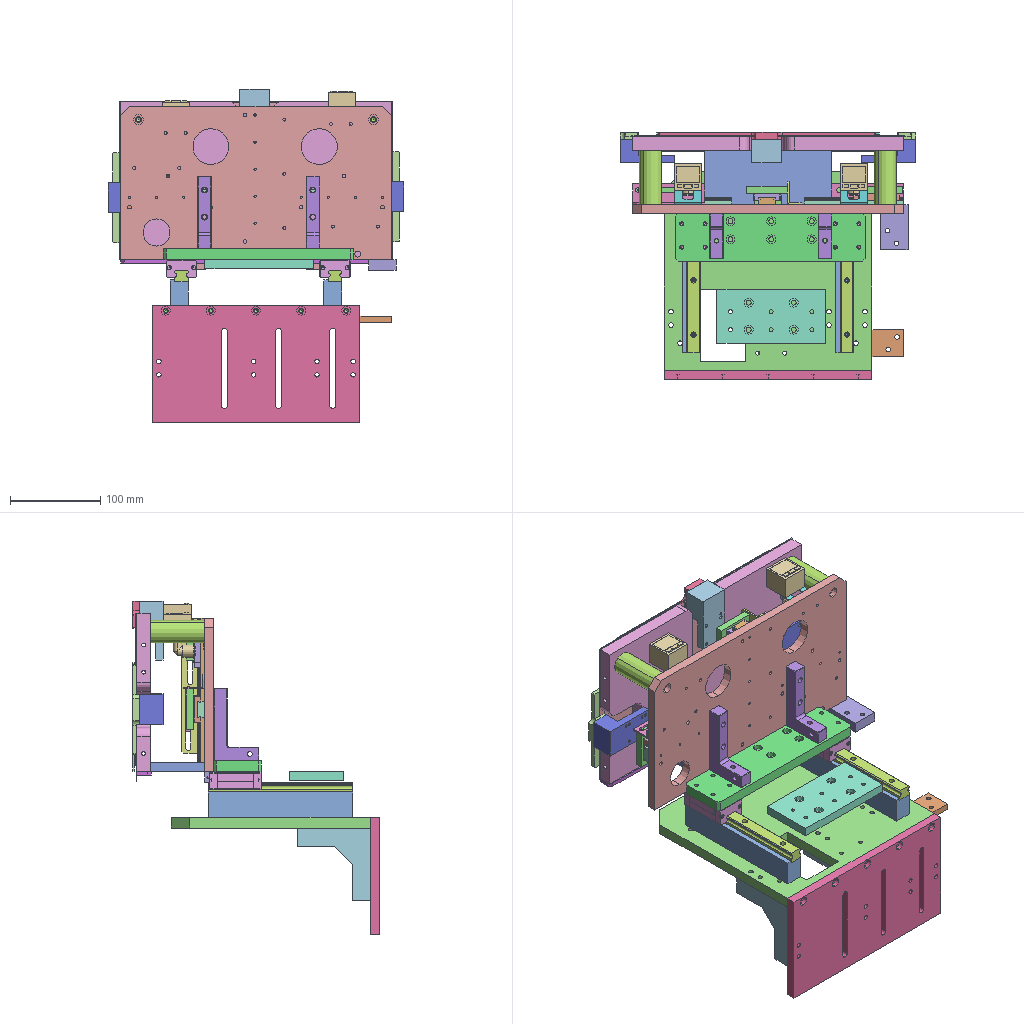Assembly | SolidWorks | 36 different items | 56 placed | box 327 x 273 x 369 mm
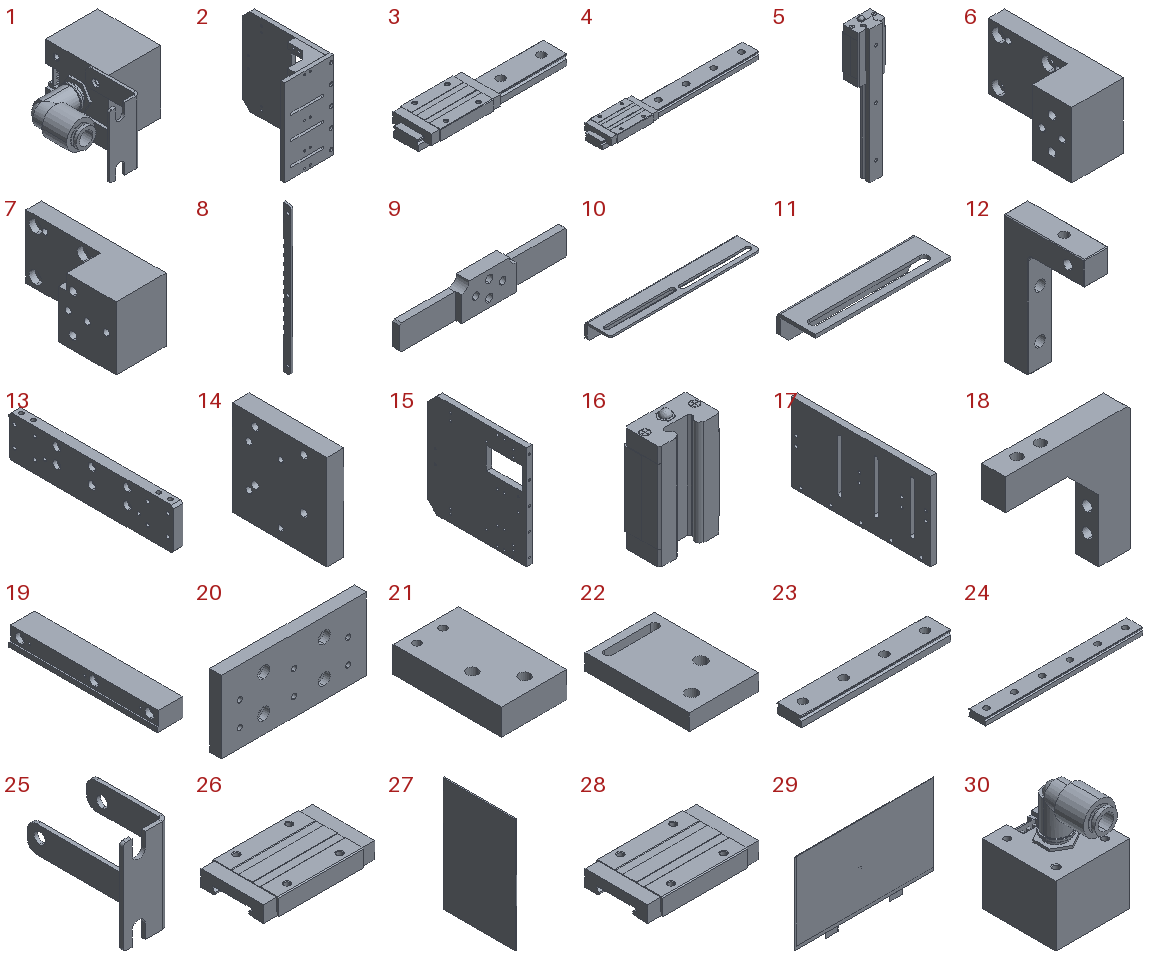Parts list (item | name | quantity | parent item | size | volume | features):
1 | (subassembly) | x2 | - | 49.1 x 45 x 30 mm | 26220 mm3 | -
2 | (subassembly) | x1 | - | 130 x 230 x 230 mm | 953540 mm3 | features LocalLPattern 2, ReferencePattern 2
3 | (subassembly) | x2 | - | 110 x 30 x 12 mm | 22408 mm3 | -
4 | (subassembly) | x1 | - | 170 x 30 x 12 mm | 29931 mm3 | -
5 | (subassembly) | x2 | - | 34 x 24 x 161.094 mm | 57035 mm3 | -
6 | - | x2 | - | 26 x 60 x 33 mm | 26587 mm3 | features HoleWzd 4, LPattern 4, ICE 2, Extrusion 1
7 | - | x1 | - | 26 x 65 x 33 mm | 33182 mm3 | features HoleWzd 4, LPattern 4, ICE 2, Extrusion 1
8 | - | x1 | - | 4 x 16 x 300 mm | 17903 mm3 | features ICE 3, Chamfer 1, Extrusion 1, LPattern 1, MirrorPattern 1
9 | - | x2 | - | 100 x 7.5 x 20 mm | 8278 mm3 | features ICE 6, Chamfer 2, LPattern 2, Cut 1, Extrusion 1, Fillet 1, HoleWzd 1
10 | - | x1 | - | 150 x 25 x 16 mm | 9935 mm3 | features ICE 4, Chamfer 3, HoleWzd 3, Extrusion 1, Fillet 1
11 | - | x2 | - | 80 x 23 x 16 mm | 4975 mm3 | features ICE 5, Chamfer 3, HoleWzd 3, Extrusion 1, Fillet 1
12 | - | x2 | - | 15 x 50 x 80 mm | 24092 mm3 | features HoleWzd 3, Chamfer 1, Extrusion 1, Fillet 1, ICE 1, LPattern 1
13 | - | x1 | - | 12 x 210 x 52.5 mm | 125690 mm3 | features LPattern 5, HoleWzd 4, ICE 2, Chamfer 1, Extrusion 1, MirrorPattern 1
14 | - | x3 | - | 8 x 45 x 45 mm | 15170 mm3 | features LPattern 5, HoleWzd 4, Extrusion 1
15 | - | x1 | in 2 | 12 x 220 x 230 mm | 548985 mm3 | features LPattern 12, HoleWzd 6, Chamfer 1, Extrusion 1, ICE 1
16 | - | x2 | in 5 | 34 x 19.4 x 59.8 mm | 30356 mm3 | features BaseBody 1
17 | - | x1 | in 2 | 10 x 230 x 130 mm | 277609 mm3 | features LPattern 6, HoleWzd 2, Extrusion 1, ICE 1
18 | - | x3 | in 2 | 80 x 15 x 80 mm | 42315 mm3 | features ICE 2, LPattern 2, Chamfer 1, Extrusion 1
19 | - | x2 | - | 28 x 160 x 20 mm | 82011 mm3 | features LPattern 3, HoleWzd 2, Extrusion 1, ICE 1
20 | - | x1 | - | 120 x 10 x 60 mm | 69123 mm3 | features HoleWzd 2, LPattern 2, Extrusion 1
21 | - | x1 | - | 30 x 50 x 12 mm | 17166 mm3 | features HoleWzd 2, Extrusion 1, LPattern 1
22 | - | x1 | - | 30 x 45 x 7 mm | 8618 mm3 | features Cut 1, Extrusion 1, HoleWzd 1
23 | - | x2 | in 3 | 110 x 18 x 7.5 mm | 13740 mm3 | features BaseBody 1, Cut 1
24 | - | x1 | in 4 | 170 x 18 x 7.5 mm | 21263 mm3 | features BaseBody 1
25 | - | x2 | in 1 | 14.5 x 44 x 30 mm | 1158 mm3 | features ICE 3, Fillet 2, EdgeFlange 1, FlatPattern 1, MirrorPattern 1, SMBaseFlange 1, SheetMetal 1
26 | - | x1 | in 4 | 50.7 x 30 x 7.8 mm | 8668 mm3 | features BaseBody 1
27 | - | x2 | - | 1.5 x 76 x 120 mm | 13680 mm3 | features Extrusion 1
28 | - | x2 | in 3 | 50.7 x 30 x 7.8 mm | 8668 mm3 | features BaseBody 1
29 | - | x1 | - | 301.97 x 1.43 x 186.39 mm | 73825 mm3 | features ICE 4, Extrusion 1, LPattern 1
30 | - | x2 | in 1 | 30 x 35.5 x 49.1 mm | 25063 mm3 | features BaseBody 1
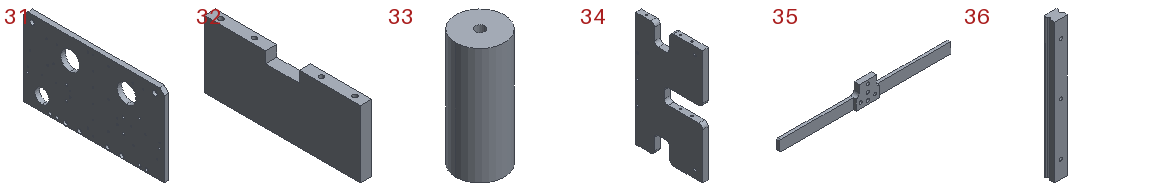31 | - | x1 | - | 10 x 300 x 170 mm | 468568 mm3 | features HoleWzd 17, LPattern 17, Cut 2, ICE 2, Chamfer 1, Extrusion 1, MirrorPattern 1
32 | - | x1 | - | 10 x 140 x 60 mm | 79757 mm3 | features HoleWzd 2, Cut 1, Extrusion 1, LPattern 1
33 | - | x2 | - | 25 x 25 x 60 mm | 28844 mm3 | features HoleWzd 2, Extrusion 1
34 | - | x1 | - | 15 x 175 x 300 mm | 650278 mm3 | features HoleWzd 10, MirrorPattern 9, LPattern 6, Cut 4, ICE 3, Fillet 2, Extrusion 1
35 | - | x1 | - | 240 x 7.5 x 30 mm | 18359 mm3 | features ICE 6, LPattern 2, Chamfer 1, Extrusion 1, Fillet 1, HoleWzd 1
36 | - | x2 | in 5 | 15 x 12.5 x 160 mm | 26679 mm3 | features BaseBody 1
Mates (type | each side: item.copy, entity, surface, feature):
In the top assembly
Coincident | 31.1 face plane Boss-Extrude 1 | 32.1 face plane Boss-Extrude 1
Coincident | 31.1 face plane Boss-Extrude 1 | 33.1 face plane Boss-Extrude 1
Coincident | 31.1 face plane Boss-Extrude 1 | 33.2 face plane Boss-Extrude 1
Coincident | 32.1 face plane Boss-Extrude 1 | 31.1 face plane Boss-Extrude 1
Parallel | 27.1 face plane Boss-Extrude 1 | 34.1 face plane Boss-Extrude 1
Coincident | 31.1 face plane Boss-Extrude 1 | 24.1 face plane Base Body 1 | 2 times
Parallel | 31.1 face plane Boss-Extrude 1 | 24.1 face plane Base Body 1
Coincident | 26.1 face plane Base Body 1 | 14.1 face plane Boss-Extrude 1
Concentric | 26.1 face cylinder Base Body 1 | 14.1 face cylinder Linear Pattern 2
Parallel | 31.1 face plane Boss-Extrude 3 | 14.1 face plane Boss-Extrude 1
DistanceDim | 35.1 face plane Boss-Extrude 1 | 34.1 face plane Boss-Extrude 1
Coincident | 32.1 face plane Boss-Extrude 1 | 34.1 face plane Boss-Extrude 1 | 2 times
Coincident | 35.1 face plane Boss-Extrude 1 | 7.1 face plane Boss-Extrude 1
DistanceDim | 24.1 face plane Base Body 1 | 31.1 face plane Boss-Extrude 3
Concentric | 35.1 face cylinder Cut-Extrude 1 | 7.1 face cylinder M4 Tapped Hole 2
Concentric | 35.1 face cylinder Linear Pattern 1 | 7.1 face cylinder Linear Pattern 3
Coincident | 14.1 face plane Boss-Extrude 1 | 10.1 face plane Boss-Extrude 1
Coincident | 31.1 face plane Boss-Extrude 1 | 10.1 face plane Boss-Extrude 1 | 2 times
Width | 27.1 face plane Boss-Extrude 1 | 27.2 face plane Boss-Extrude 1 | 34.1 face plane Boss-Extrude 1 | 34.1 face plane Boss-Extrude 1
DistanceDim | 34.1 face plane Boss-Extrude 1 | 31.1 face plane Boss-Extrude 3
Coincident | 34.1 face plane Boss-Extrude 1 | 8.1 face plane Boss-Extrude 1 | 3 times
Parallel | 34.1 face plane Boss-Extrude 1 | 8.1 face plane Boss-Extrude 1
Coincident | 31.1 face plane Boss-Extrude 1 | 23.1 face plane Base Body 1
DistanceDim | 23.1 face plane Base Body 1 | 31.1 face plane Boss-Extrude 1
Coincident | 31.1 face plane Boss-Extrude 3 | 23.1 face plane Base Body 1
Coincident | 28.1 face plane Base Body 1 | 14.2 face plane Boss-Extrude 1
Concentric | 28.1 face cylinder Base Body 1 | 14.2 face cylinder Linear Pattern 1
Parallel | 28.1 face plane Base Body 1 | 14.2 face plane Boss-Extrude 1
Coincident | 31.1 face plane Boss-Extrude 1 | 23.2 face plane Base Body 1
Coincident | 31.1 face plane Boss-Extrude 3 | 23.2 face plane Base Body 1
Coincident | 23.1 face plane Base Body 1 | 23.2 face plane Base Body 1
Coincident | 28.2 face plane Base Body 1 | 14.3 face plane Boss-Extrude 1
Concentric | 28.2 face cylinder Base Body 1 | 14.3 face cylinder M3 Hex Socket Cap Screw Counterbore 1
Parallel | 28.2 face plane Base Body 1 | 14.3 face plane Boss-Extrude 1
Coincident | 6.1 face plane Boss-Extrude 2 | 9.1 face plane Boss-Extrude 3
Concentric | 6.1 face cylinder Linear Pattern 2 | 9.1 face cylinder Linear Pattern 1
Concentric | 6.1 face cylinder M4 Tapped Hole 2 | 9.1 face cylinder Linear Pattern 1
Coincident | 6.2 face plane Boss-Extrude 2 | 9.2 face plane Boss-Extrude 3
Concentric | 6.2 face cylinder Linear Pattern 2 | 9.2 face cylinder Linear Pattern 1
Concentric | 6.2 face cylinder M4 Tapped Hole 2 | 9.2 face cylinder Linear Pattern 1
Coincident | 14.2 face plane Boss-Extrude 1 | 11.1 face plane Boss-Extrude 1
Coincident | 31.1 face plane Boss-Extrude 1 | 11.1 face plane Boss-Extrude 1
Coincident | 31.1 face plane Boss-Extrude 3 | 11.1 face plane Boss-Extrude 1
Coincident | 14.3 face plane Boss-Extrude 1 | 11.2 face plane Boss-Extrude 1
Coincident | 31.1 face plane Boss-Extrude 1 | 11.2 face plane Boss-Extrude 1
Coincident | 31.1 face plane Boss-Extrude 3 | 11.2 face plane Boss-Extrude 1
Coincident | 31.1 face plane Boss-Extrude 1 | 25.1 face plane Edge Flange 1
Coincident | 12.1 face plane Boss-Extrude 1 | 13.1 face plane Boss-Extrude 1
DistanceDim | 12.1 face plane Boss-Extrude 1 | 13.1 face plane Boss-Extrude 2
Coincident | 31.1 face plane Boss-Extrude 1 | 13.1 face plane Boss-Extrude 1 | 2 times
Coincident | 31.1 face plane Boss-Extrude 1 | 12.2 face plane Boss-Extrude 1
Parallel | 31.1 face plane Boss-Extrude 1 | 6.2 face plane Boss-Extrude 1
DistanceDim | 6.2 face plane Boss-Extrude 1 | 31.1 face plane Boss-Extrude 1
DistanceDim | 6.1 face plane Boss-Extrude 1 | 31.1 face plane Boss-Extrude 1
Parallel | 14.1 face plane Boss-Extrude 1 | 7.1 face plane Boss-Extrude 1
Coincident | 34.1 face plane Boss-Extrude 1 | 29.1 face plane Boss-Extrude 1 | 2 times
Width | 29.1 face plane Boss-Extrude 1 | 29.1 face plane Boss-Extrude 1 | 34.1 face plane Boss-Extrude 1 | 34.1 face plane Boss-Extrude 1
Coincident | 19.1 face plane Cut-Extrude 1 | 36.1 face plane Base Body 1 | 2 times
Coincident | 19.1 face plane Boss-Extrude 1 | 36.1 face plane Base Body 1
DistanceDim | 13.1 face plane Boss-Extrude 2 | 31.1 face plane Boss-Extrude 3
Width | 32.1 face plane Boss-Extrude 1 | 32.1 face plane Boss-Extrude 1 | 31.1 face plane Boss-Extrude 3 | 31.1 face plane Boss-Extrude 3
Parallel | 31.1 face plane Boss-Extrude 1 | 25.1 face plane Base Flange 1
Concentric | 33.1 face cylinder M6 Tapped Hole 2 | 34.1 face cylinder M6 Socket Head Cap Screw Counterbore 1
Concentric | 33.2 face cylinder M6 Tapped Hole 2 | 34.1 face cylinder Mirror 5
Coincident | 31.1 face plane Boss-Extrude 1 | 21.1 face plane Boss-Extrude 1
Concentric | 31.1 face cylinder M3 Tapped Hole 4 | 21.1 face cylinder Linear Pattern 1
Concentric | 31.1 face cylinder M3 Tapped Hole 4 | 21.1 face cylinder M3 Socket Head Cap Screw Counterbore 1
Coincident | 19.2 face plane Boss-Extrude 1 | 15.1 face plane Boss-Extrude 1
Concentric | 19.2 face cylinder Linear Pattern 2 | 15.1 face cylinder Linear Pattern 12
Concentric | 19.1 face cylinder Linear Pattern 2 | 15.1 face cylinder Linear Pattern 11
Coincident | 22.1 face plane Boss-Extrude 1 | 15.1 face plane Boss-Extrude 1
Concentric | 22.1 face cylinder Cut-Extrude 1 | 15.1 face cylinder M3 Tapped Hole 1
Parallel | 22.1 face plane Boss-Extrude 1 | 17.1 face plane Boss-Extrude 1
Concentric | 13.1 face cylinder Linear Pattern 4 | 16.1 face cylinder Base Body 1
Concentric | 13.1 face cylinder Linear Pattern 4 | 16.1 face cone Base Body 1
DistanceDim | 25.1 face plane Edge Flange 1 | 31.1 face plane Boss-Extrude 3
Coincident | 31.1 face plane Boss-Extrude 1 | 25.2 face plane Edge Flange 1
DistanceDim | 30.1 face plane Base Body 1 | 31.1 face plane Boss-Extrude 1
DistanceDim | 25.2 face plane Edge Flange 1 | 31.1 face plane Boss-Extrude 3
In subassembly 4
DistanceDim | 26.2 face plane Base Body 1 | 24.2 face plane Base Body 1
Width | 26.2 face plane Base Body 1 | 26.2 face plane Base Body 1 | 24.2 face plane Base Body 1 | 24.2 face plane Base Body 1
In subassembly 3
DistanceDim | 28.3 face plane Base Body 1 | 23.3 face plane Base Body 1
Width | 28.3 face plane Base Body 1 | 28.3 face plane Base Body 1 | 23.3 face plane Base Body 1 | 23.3 face plane Base Body 1
In subassembly 1
Concentric | 25.3 face cylinder Cut-Extrude 3 | 30.2 face cylinder Base Body 1 | 2 times
Coincident | 25.3 face plane Base Flange 1 | 30.2 face plane Base Body 1
In subassembly 5
Concentric | 36.2 face cylinder Base Body 1 | 16.2 face cylinder Base Body 1 | 2 times
LimitDistanceDim | 16.2 face plane Base Body 1 | 36.2 face plane Base Body 1
In subassembly 2
Coincident | 15.2 face plane Boss-Extrude 1 | 17.2 face plane Boss-Extrude 1 | 3 times
Coincident | 15.2 face plane Boss-Extrude 1 | 18.1 face plane Boss-Extrude 1
Coincident | 17.2 face plane Boss-Extrude 1 | 18.1 face plane Boss-Extrude 1
DistanceDim | 15.2 face plane Boss-Extrude 1 | 18.1 face plane Boss-Extrude 1